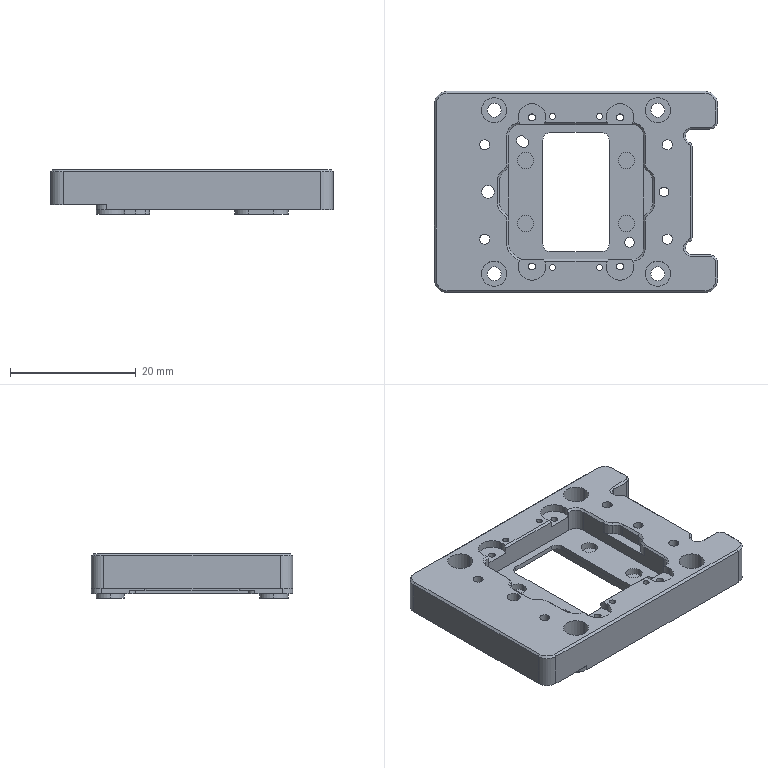Part | 1 solid | 404 faces | box 45 x 32 x 7.05 mm | volume 5335 mm3 | plane 162 | cylinder 139 | spline 78 | cone 25 | commonest cylinder face diameters 2 x16 4 x12 4.4 x12 4.5 x12 2.2 x10 3.4 x10